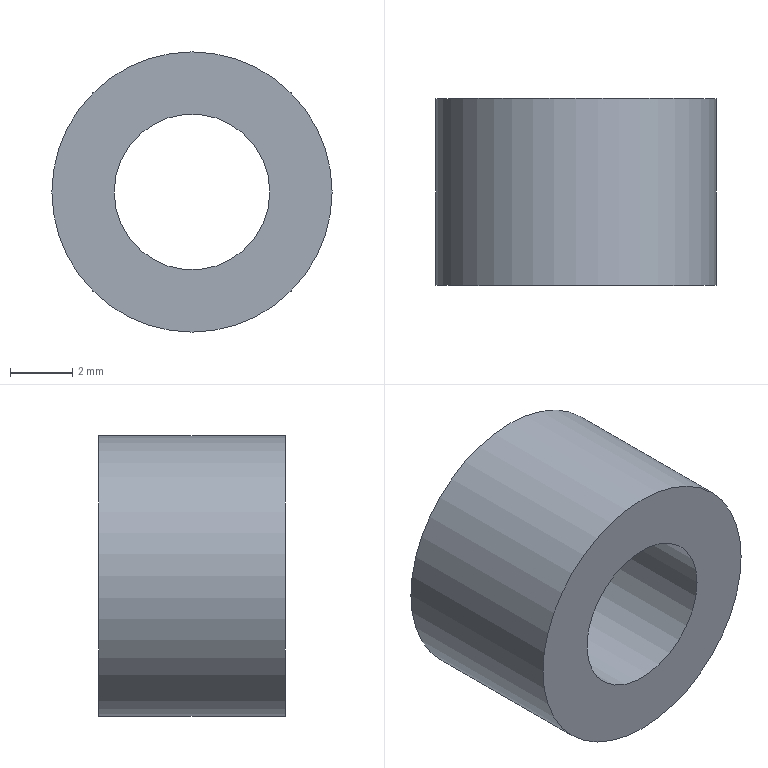Part | STEP file | 1-69.3 | 1 solid | 4 faces | box 9 x 6 x 9 mm | volume 263.894 mm3 | plane 2 | cylinder 2 | commonest cylinder face diameters 5 x1 9 x1
STEP:
#1=CARTESIAN_POINT('',(0.,0.,0.));
#2=DIRECTION('',(0.,0.,1.));
#3=DIRECTION('',(1.,0.,0.));
#4=AXIS2_PLACEMENT_3D('',#1,#2,#3);
#5=CARTESIAN_POINT('',(4.5,-3.,0.));
#6=VERTEX_POINT('',#5);
#7=CARTESIAN_POINT('',(0.,-3.,0.));
#8=DIRECTION('',(0.,-1.,0.));
#9=DIRECTION('',(1.,0.,0.));
#10=AXIS2_PLACEMENT_3D('',#7,#8,#9);
#11=CIRCLE('',#10,4.5);
#12=CARTESIAN_POINT('',(-1.206,-3.,0.));
#13=DIRECTION('',(0.,-1.,0.));
#14=DIRECTION('',(1.,0.,0.));
#15=AXIS2_PLACEMENT_3D('',#12,#13,#14);
#16=PLANE('',#15);
#17=CARTESIAN_POINT('',(1.206,0.));
#18=DIRECTION('',(1.,0.));
#19=AXIS2_PLACEMENT_2D('',#17,#18);
#20=CIRCLE('',#19,4.5);
#21=(GEOMETRIC_REPRESENTATION_CONTEXT(2)PARAMETRIC_REPRESENTATION_CONTEXT()REPRESENTATION_CONTEXT('',''));
#22=DEFINITIONAL_REPRESENTATION('',(#20),#21);
#23=PCURVE('',#16,#22);
#24=CARTESIAN_POINT('',(0.,-3.,0.));
#25=DIRECTION('',(0.,1.,0.));
#26=DIRECTION('',(1.,0.,0.));
#27=AXIS2_PLACEMENT_3D('',#24,#25,#26);
#28=CYLINDRICAL_SURFACE('',#27,4.5);
#29=CARTESIAN_POINT('',(6.283,0.));
#30=DIRECTION('',(-1.,0.));
#31=VECTOR('',#30,1.);
#32=LINE('',#29,#31);
#33=(GEOMETRIC_REPRESENTATION_CONTEXT(2)PARAMETRIC_REPRESENTATION_CONTEXT()REPRESENTATION_CONTEXT('',''));
#34=DEFINITIONAL_REPRESENTATION('',(#32),#33);
#35=PCURVE('',#28,#34);
#36=SURFACE_CURVE('',#11,(#23,#35),.PCURVE_S1.);
#37=EDGE_CURVE('',#6,#6,#36,.T.);
#38=ORIENTED_EDGE('',*,*,#37,.T.);
#39=EDGE_LOOP('',(#38));
#40=FACE_BOUND('',#39,.T.);
#41=CARTESIAN_POINT('',(2.5,-3.,0.));
#42=VERTEX_POINT('',#41);
#43=CARTESIAN_POINT('',(0.,-3.,0.));
#44=DIRECTION('',(0.,1.,0.));
#45=DIRECTION('',(1.,0.,0.));
#46=AXIS2_PLACEMENT_3D('',#43,#44,#45);
#47=CIRCLE('',#46,2.5);
#48=CARTESIAN_POINT('',(3.706,0.));
#49=CARTESIAN_POINT('',(3.706,-4.33));
#50=CARTESIAN_POINT('',(-0.04423,-2.165));
#51=CARTESIAN_POINT('',(-3.794,0.));
#52=CARTESIAN_POINT('',(-0.04423,2.165));
#53=CARTESIAN_POINT('',(3.706,4.33));
#54=CARTESIAN_POINT('',(3.706,0.));
#55=(BOUNDED_CURVE()B_SPLINE_CURVE(2,(#48,#49,#50,#51,#52,#53,#54),.UNSPECIFIED.,.T.,.F.)B_SPLINE_CURVE_WITH_KNOTS((1,2,2,2,2,1),(-2.094,0.,2.094,4.189,6.283,8.378),.UNSPECIFIED.)CURVE()GEOMETRIC_REPRESENTATION_ITEM()RATIONAL_B_SPLINE_CURVE((1.,0.5,1.,0.5,1.,0.5,1.))REPRESENTATION_ITEM(''));
#56=(GEOMETRIC_REPRESENTATION_CONTEXT(2)PARAMETRIC_REPRESENTATION_CONTEXT()REPRESENTATION_CONTEXT('',''));
#57=DEFINITIONAL_REPRESENTATION('',(#55),#56);
#58=PCURVE('',#16,#57);
#59=CARTESIAN_POINT('',(0.,-3.,0.));
#60=DIRECTION('',(0.,1.,0.));
#61=DIRECTION('',(1.,0.,0.));
#62=AXIS2_PLACEMENT_3D('',#59,#60,#61);
#63=CYLINDRICAL_SURFACE('',#62,2.5);
#64=CARTESIAN_POINT('',(0.,0.));
#65=DIRECTION('',(1.,0.));
#66=VECTOR('',#65,1.);
#67=LINE('',#64,#66);
#68=(GEOMETRIC_REPRESENTATION_CONTEXT(2)PARAMETRIC_REPRESENTATION_CONTEXT()REPRESENTATION_CONTEXT('',''));
#69=DEFINITIONAL_REPRESENTATION('',(#67),#68);
#70=PCURVE('',#63,#69);
#71=SURFACE_CURVE('',#47,(#58,#70),.PCURVE_S1.);
#72=EDGE_CURVE('',#42,#42,#71,.T.);
#73=ORIENTED_EDGE('',*,*,#72,.T.);
#74=EDGE_LOOP('',(#73));
#75=FACE_BOUND('',#74,.T.);
#76=ADVANCED_FACE('',(#40,#75),#16,.T.);
#77=CARTESIAN_POINT('',(4.5,3.,0.));
#78=VERTEX_POINT('',#77);
#79=CARTESIAN_POINT('',(0.,3.,0.));
#80=DIRECTION('',(0.,-1.,0.));
#81=DIRECTION('',(1.,0.,0.));
#82=AXIS2_PLACEMENT_3D('',#79,#80,#81);
#83=CIRCLE('',#82,4.5);
#84=CARTESIAN_POINT('',(-1.206,3.,0.));
#85=DIRECTION('',(0.,-1.,0.));
#86=DIRECTION('',(1.,0.,0.));
#87=AXIS2_PLACEMENT_3D('',#84,#85,#86);
#88=PLANE('',#87);
#89=CARTESIAN_POINT('',(1.206,0.));
#90=DIRECTION('',(1.,0.));
#91=AXIS2_PLACEMENT_2D('',#89,#90);
#92=CIRCLE('',#91,4.5);
#93=(GEOMETRIC_REPRESENTATION_CONTEXT(2)PARAMETRIC_REPRESENTATION_CONTEXT()REPRESENTATION_CONTEXT('',''));
#94=DEFINITIONAL_REPRESENTATION('',(#92),#93);
#95=PCURVE('',#88,#94);
#96=CARTESIAN_POINT('',(6.283,6.));
#97=DIRECTION('',(-1.,0.));
#98=VECTOR('',#97,1.);
#99=LINE('',#96,#98);
#100=(GEOMETRIC_REPRESENTATION_CONTEXT(2)PARAMETRIC_REPRESENTATION_CONTEXT()REPRESENTATION_CONTEXT('',''));
#101=DEFINITIONAL_REPRESENTATION('',(#99),#100);
#102=PCURVE('',#28,#101);
#103=SURFACE_CURVE('',#83,(#95,#102),.PCURVE_S1.);
#104=EDGE_CURVE('',#78,#78,#103,.T.);
#105=ORIENTED_EDGE('',*,*,#104,.T.);
#106=EDGE_LOOP('',(#105));
#107=FACE_BOUND('',#106,.F.);
#108=CARTESIAN_POINT('',(2.5,3.,0.));
#109=VERTEX_POINT('',#108);
#110=CARTESIAN_POINT('',(0.,3.,0.));
#111=DIRECTION('',(0.,1.,0.));
#112=DIRECTION('',(1.,0.,0.));
#113=AXIS2_PLACEMENT_3D('',#110,#111,#112);
#114=CIRCLE('',#113,2.5);
#115=CARTESIAN_POINT('',(3.706,0.));
#116=CARTESIAN_POINT('',(3.706,-4.33));
#117=CARTESIAN_POINT('',(-0.04423,-2.165));
#118=CARTESIAN_POINT('',(-3.794,0.));
#119=CARTESIAN_POINT('',(-0.04423,2.165));
#120=CARTESIAN_POINT('',(3.706,4.33));
#121=CARTESIAN_POINT('',(3.706,0.));
#122=(BOUNDED_CURVE()B_SPLINE_CURVE(2,(#115,#116,#117,#118,#119,#120,#121),.UNSPECIFIED.,.T.,.F.)B_SPLINE_CURVE_WITH_KNOTS((1,2,2,2,2,1),(-2.094,0.,2.094,4.189,6.283,8.378),.UNSPECIFIED.)CURVE()GEOMETRIC_REPRESENTATION_ITEM()RATIONAL_B_SPLINE_CURVE((1.,0.5,1.,0.5,1.,0.5,1.))REPRESENTATION_ITEM(''));
#123=(GEOMETRIC_REPRESENTATION_CONTEXT(2)PARAMETRIC_REPRESENTATION_CONTEXT()REPRESENTATION_CONTEXT('',''));
#124=DEFINITIONAL_REPRESENTATION('',(#122),#123);
#125=PCURVE('',#88,#124);
#126=CARTESIAN_POINT('',(0.,6.));
#127=DIRECTION('',(1.,0.));
#128=VECTOR('',#127,1.);
#129=LINE('',#126,#128);
#130=(GEOMETRIC_REPRESENTATION_CONTEXT(2)PARAMETRIC_REPRESENTATION_CONTEXT()REPRESENTATION_CONTEXT('',''));
#131=DEFINITIONAL_REPRESENTATION('',(#129),#130);
#132=PCURVE('',#63,#131);
#133=SURFACE_CURVE('',#114,(#125,#132),.PCURVE_S1.);
#134=EDGE_CURVE('',#109,#109,#133,.T.);
#135=ORIENTED_EDGE('',*,*,#134,.T.);
#136=EDGE_LOOP('',(#135));
#137=FACE_BOUND('',#136,.F.);
#138=ADVANCED_FACE('',(#107,#137),#88,.F.);
#139=CARTESIAN_POINT('',(4.5,-3.,0.));
#140=DIRECTION('',(0.,1.,0.));
#141=VECTOR('',#140,1.);
#142=LINE('',#139,#141);
#143=CARTESIAN_POINT('',(6.283,0.));
#144=DIRECTION('',(0.,1.));
#145=VECTOR('',#144,1.);
#146=LINE('',#143,#145);
#147=(GEOMETRIC_REPRESENTATION_CONTEXT(2)PARAMETRIC_REPRESENTATION_CONTEXT()REPRESENTATION_CONTEXT('',''));
#148=DEFINITIONAL_REPRESENTATION('',(#146),#147);
#149=PCURVE('',#28,#148);
#150=CARTESIAN_POINT('',(0.,0.));
#151=DIRECTION('',(0.,1.));
#152=VECTOR('',#151,1.);
#153=LINE('',#150,#152);
#154=(GEOMETRIC_REPRESENTATION_CONTEXT(2)PARAMETRIC_REPRESENTATION_CONTEXT()REPRESENTATION_CONTEXT('',''));
#155=DEFINITIONAL_REPRESENTATION('',(#153),#154);
#156=PCURVE('',#28,#155);
#157=SEAM_CURVE('',#142,(#149,#156),.PCURVE_S1.);
#158=EDGE_CURVE('',#6,#78,#157,.T.);
#159=ORIENTED_EDGE('',*,*,#158,.T.);
#160=ORIENTED_EDGE('',*,*,#104,.T.);
#161=ORIENTED_EDGE('',*,*,#158,.F.);
#162=ORIENTED_EDGE('',*,*,#37,.F.);
#163=EDGE_LOOP('',(#159,#160,#161,#162));
#164=FACE_BOUND('',#163,.T.);
#165=ADVANCED_FACE('',(#164),#28,.T.);
#166=ORIENTED_EDGE('',*,*,#72,.T.);
#167=CARTESIAN_POINT('',(2.5,-3.,0.));
#168=DIRECTION('',(0.,1.,0.));
#169=VECTOR('',#168,1.);
#170=LINE('',#167,#169);
#171=CARTESIAN_POINT('',(6.283,0.));
#172=DIRECTION('',(0.,1.));
#173=VECTOR('',#172,1.);
#174=LINE('',#171,#173);
#175=(GEOMETRIC_REPRESENTATION_CONTEXT(2)PARAMETRIC_REPRESENTATION_CONTEXT()REPRESENTATION_CONTEXT('',''));
#176=DEFINITIONAL_REPRESENTATION('',(#174),#175);
#177=PCURVE('',#63,#176);
#178=CARTESIAN_POINT('',(0.,0.));
#179=DIRECTION('',(0.,1.));
#180=VECTOR('',#179,1.);
#181=LINE('',#178,#180);
#182=(GEOMETRIC_REPRESENTATION_CONTEXT(2)PARAMETRIC_REPRESENTATION_CONTEXT()REPRESENTATION_CONTEXT('',''));
#183=DEFINITIONAL_REPRESENTATION('',(#181),#182);
#184=PCURVE('',#63,#183);
#185=SEAM_CURVE('',#170,(#177,#184),.PCURVE_S1.);
#186=EDGE_CURVE('',#42,#109,#185,.T.);
#187=ORIENTED_EDGE('',*,*,#186,.T.);
#188=ORIENTED_EDGE('',*,*,#134,.F.);
#189=ORIENTED_EDGE('',*,*,#186,.F.);
#190=EDGE_LOOP('',(#166,#187,#188,#189));
#191=FACE_BOUND('',#190,.F.);
#192=ADVANCED_FACE('',(#191),#63,.F.);
#193=CLOSED_SHELL('',(#76,#138,#165,#192));
#194=MANIFOLD_SOLID_BREP('',#193);
#195=(LENGTH_UNIT()NAMED_UNIT(*)SI_UNIT(.MILLI.,.METRE.));
#196=UNCERTAINTY_MEASURE_WITH_UNIT(LENGTH_MEASURE(0.0000001),#195,'','');
#197=(NAMED_UNIT(*)PLANE_ANGLE_UNIT()SI_UNIT($,.RADIAN.));
#198=(NAMED_UNIT(*)SI_UNIT($,.STERADIAN.)SOLID_ANGLE_UNIT());
#199=(GEOMETRIC_REPRESENTATION_CONTEXT(3)GLOBAL_UNCERTAINTY_ASSIGNED_CONTEXT((#196))GLOBAL_UNIT_ASSIGNED_CONTEXT((#195,#197,#198))REPRESENTATION_CONTEXT('',''));
#200=ADVANCED_BREP_SHAPE_REPRESENTATION('',(#4,#194),#199);